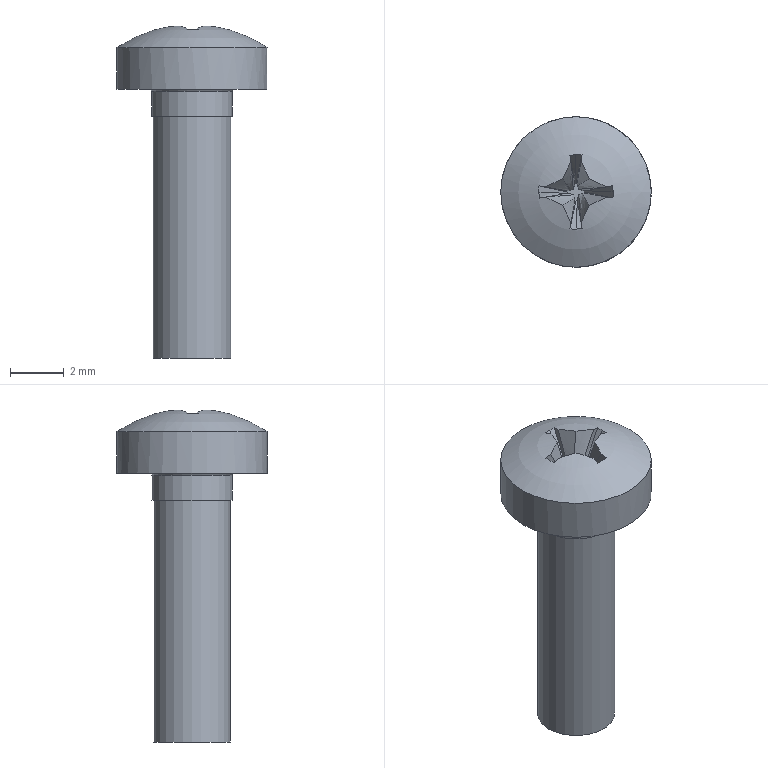Part | NX | features SKETCH 3, DATUM_CSYS 2, DATUM_PLANE 2, FSET 1, LINE 1, META 1, SKIN 1, SWP104 1, SYMBOLIC_THREAD 1, THREADS 1 | 1 solid | 33 faces | box 5.6 x 5.6 x 12.351 mm | volume 111.736 mm3 | spline 20 | plane 8 | cylinder 3 | sphere 1 | torus 1 | commonest cylinder face diameters 2.874 x1 3 x1 5.6 x1
STEP:
#1=CARTESIAN_POINT('',(-2.8,0.,1.542));
#2=VERTEX_POINT('',#1);
#3=CARTESIAN_POINT('',(0.,0.,1.542));
#4=DIRECTION('',(0.,0.,-1.));
#5=DIRECTION('',(-1.,0.,0.));
#6=AXIS2_PLACEMENT_3D('',#3,#4,#5);
#7=CIRCLE('',#6,2.8);
#8=EDGE_CURVE('',#2,#2,#7,.T.);
#9=ORIENTED_EDGE('',*,*,#8,.F.);
#10=EDGE_LOOP('',(#9));
#11=FACE_BOUND('',#10,.T.);
#12=CARTESIAN_POINT('',(-0.4967,0.4916,2.351));
#13=VERTEX_POINT('',#12);
#14=CARTESIAN_POINT('',(-1.137,0.1895,2.265));
#15=VERTEX_POINT('',#14);
#16=CARTESIAN_POINT('',(-0.4967,0.4916,2.351));
#17=CARTESIAN_POINT('',(-0.7133,0.3939,2.339));
#18=CARTESIAN_POINT('',(-0.9272,0.2926,2.31));
#19=CARTESIAN_POINT('',(-1.137,0.1895,2.265));
#20=B_SPLINE_CURVE_WITH_KNOTS('',3,(#16,#17,#18,#19),.UNSPECIFIED.,.F.,.F.,(4,4),(0.,0.0007137),.UNSPECIFIED.);
#21=EDGE_CURVE('',#13,#15,#20,.T.);
#22=ORIENTED_EDGE('',*,*,#21,.F.);
#23=CARTESIAN_POINT('',(-0.1932,1.124,2.268));
#24=VERTEX_POINT('',#23);
#25=CARTESIAN_POINT('',(-0.1932,1.124,2.268));
#26=CARTESIAN_POINT('',(-0.2989,0.9182,2.312));
#27=CARTESIAN_POINT('',(-0.3995,0.7062,2.339));
#28=CARTESIAN_POINT('',(-0.4967,0.4916,2.351));
#29=B_SPLINE_CURVE_WITH_KNOTS('',3,(#25,#26,#27,#28),.UNSPECIFIED.,.F.,.F.,(4,4),(0.,0.0007074),.UNSPECIFIED.);
#30=EDGE_CURVE('',#24,#13,#29,.T.);
#31=ORIENTED_EDGE('',*,*,#30,.F.);
#32=CARTESIAN_POINT('',(-0.2285,1.371,2.203));
#33=VERTEX_POINT('',#32);
#34=CARTESIAN_POINT('',(-0.2285,1.371,2.203));
#35=CARTESIAN_POINT('',(-0.2178,1.289,2.227));
#36=CARTESIAN_POINT('',(-0.2059,1.207,2.249));
#37=CARTESIAN_POINT('',(-0.1932,1.124,2.268));
#38=B_SPLINE_CURVE_WITH_KNOTS('',3,(#34,#35,#36,#37),.UNSPECIFIED.,.F.,.F.,(4,4),(0.,0.0002572),.UNSPECIFIED.);
#39=EDGE_CURVE('',#33,#24,#38,.T.);
#40=ORIENTED_EDGE('',*,*,#39,.F.);
#41=CARTESIAN_POINT('',(-0.005049,1.379,2.206));
#42=VERTEX_POINT('',#41);
#43=CARTESIAN_POINT('',(-0.005049,1.379,2.206));
#44=CARTESIAN_POINT('',(-0.07956,1.377,2.207));
#45=CARTESIAN_POINT('',(-0.1541,1.374,2.205));
#46=CARTESIAN_POINT('',(-0.2285,1.371,2.203));
#47=B_SPLINE_CURVE_WITH_KNOTS('',3,(#43,#44,#45,#46),.UNSPECIFIED.,.F.,.F.,(4,4),(0.,0.0002236),.UNSPECIFIED.);
#48=EDGE_CURVE('',#42,#33,#47,.T.);
#49=ORIENTED_EDGE('',*,*,#48,.F.);
#50=CARTESIAN_POINT('',(0.2242,1.376,2.202));
#51=VERTEX_POINT('',#50);
#52=CARTESIAN_POINT('',(0.,-1.169,-1.87));
#53=DIRECTION('',(0.,-0.848,0.53));
#54=DIRECTION('',(0.,-0.53,-0.848));
#55=AXIS2_PLACEMENT_3D('',#52,#53,#54);
#56=CIRCLE('',#55,4.806);
#57=EDGE_CURVE('',#51,#42,#56,.T.);
#58=ORIENTED_EDGE('',*,*,#57,.F.);
#59=CARTESIAN_POINT('',(0.1895,1.137,2.265));
#60=VERTEX_POINT('',#59);
#61=CARTESIAN_POINT('',(0.1895,1.137,2.265));
#62=CARTESIAN_POINT('',(0.2017,1.217,2.246));
#63=CARTESIAN_POINT('',(0.2134,1.297,2.225));
#64=CARTESIAN_POINT('',(0.2242,1.376,2.202));
#65=B_SPLINE_CURVE_WITH_KNOTS('',3,(#61,#62,#63,#64),.UNSPECIFIED.,.F.,.F.,(4,4),(0.,0.0002499),.UNSPECIFIED.);
#66=EDGE_CURVE('',#60,#51,#65,.T.);
#67=ORIENTED_EDGE('',*,*,#66,.F.);
#68=CARTESIAN_POINT('',(0.4916,0.4967,2.351));
#69=VERTEX_POINT('',#68);
#70=CARTESIAN_POINT('',(0.4916,0.4967,2.351));
#71=CARTESIAN_POINT('',(0.3939,0.7133,2.339));
#72=CARTESIAN_POINT('',(0.2926,0.9272,2.31));
#73=CARTESIAN_POINT('',(0.1895,1.137,2.265));
#74=B_SPLINE_CURVE_WITH_KNOTS('',3,(#70,#71,#72,#73),.UNSPECIFIED.,.F.,.F.,(4,4),(0.,0.0007137),.UNSPECIFIED.);
#75=EDGE_CURVE('',#69,#60,#74,.T.);
#76=ORIENTED_EDGE('',*,*,#75,.F.);
#77=CARTESIAN_POINT('',(1.124,0.1932,2.268));
#78=VERTEX_POINT('',#77);
#79=CARTESIAN_POINT('',(1.124,0.1932,2.268));
#80=CARTESIAN_POINT('',(0.9182,0.2989,2.312));
#81=CARTESIAN_POINT('',(0.7062,0.3995,2.339));
#82=CARTESIAN_POINT('',(0.4916,0.4967,2.351));
#83=B_SPLINE_CURVE_WITH_KNOTS('',3,(#79,#80,#81,#82),.UNSPECIFIED.,.F.,.F.,(4,4),(0.,0.0007074),.UNSPECIFIED.);
#84=EDGE_CURVE('',#78,#69,#83,.T.);
#85=ORIENTED_EDGE('',*,*,#84,.F.);
#86=CARTESIAN_POINT('',(1.371,0.2285,2.203));
#87=VERTEX_POINT('',#86);
#88=CARTESIAN_POINT('',(1.371,0.2285,2.203));
#89=CARTESIAN_POINT('',(1.289,0.2178,2.227));
#90=CARTESIAN_POINT('',(1.207,0.2059,2.249));
#91=CARTESIAN_POINT('',(1.124,0.1932,2.268));
#92=B_SPLINE_CURVE_WITH_KNOTS('',3,(#88,#89,#90,#91),.UNSPECIFIED.,.F.,.F.,(4,4),(0.,0.0002572),.UNSPECIFIED.);
#93=EDGE_CURVE('',#87,#78,#92,.T.);
#94=ORIENTED_EDGE('',*,*,#93,.F.);
#95=CARTESIAN_POINT('',(1.379,0.005049,2.206));
#96=VERTEX_POINT('',#95);
#97=CARTESIAN_POINT('',(1.379,0.005049,2.206));
#98=CARTESIAN_POINT('',(1.377,0.07956,2.207));
#99=CARTESIAN_POINT('',(1.374,0.1541,2.205));
#100=CARTESIAN_POINT('',(1.371,0.2285,2.203));
#101=B_SPLINE_CURVE_WITH_KNOTS('',3,(#97,#98,#99,#100),.UNSPECIFIED.,.F.,.F.,(4,4),(0.,0.0002236),.UNSPECIFIED.);
#102=EDGE_CURVE('',#96,#87,#101,.T.);
#103=ORIENTED_EDGE('',*,*,#102,.F.);
#104=CARTESIAN_POINT('',(1.376,-0.2242,2.202));
#105=VERTEX_POINT('',#104);
#106=CARTESIAN_POINT('',(-1.169,0.,-1.87));
#107=DIRECTION('',(-0.848,0.,0.53));
#108=DIRECTION('',(0.53,0.,0.848));
#109=AXIS2_PLACEMENT_3D('',#106,#107,#108);
#110=CIRCLE('',#109,4.806);
#111=EDGE_CURVE('',#105,#96,#110,.T.);
#112=ORIENTED_EDGE('',*,*,#111,.F.);
#113=CARTESIAN_POINT('',(1.137,-0.1895,2.265));
#114=VERTEX_POINT('',#113);
#115=CARTESIAN_POINT('',(1.137,-0.1895,2.265));
#116=CARTESIAN_POINT('',(1.217,-0.2017,2.246));
#117=CARTESIAN_POINT('',(1.297,-0.2134,2.225));
#118=CARTESIAN_POINT('',(1.376,-0.2242,2.202));
#119=B_SPLINE_CURVE_WITH_KNOTS('',3,(#115,#116,#117,#118),.UNSPECIFIED.,.F.,.F.,(4,4),(0.,0.0002499),.UNSPECIFIED.);
#120=EDGE_CURVE('',#114,#105,#119,.T.);
#121=ORIENTED_EDGE('',*,*,#120,.F.);
#122=CARTESIAN_POINT('',(0.4967,-0.4916,2.351));
#123=VERTEX_POINT('',#122);
#124=CARTESIAN_POINT('',(0.4967,-0.4916,2.351));
#125=CARTESIAN_POINT('',(0.7133,-0.3939,2.339));
#126=CARTESIAN_POINT('',(0.9272,-0.2926,2.31));
#127=CARTESIAN_POINT('',(1.137,-0.1895,2.265));
#128=B_SPLINE_CURVE_WITH_KNOTS('',3,(#124,#125,#126,#127),.UNSPECIFIED.,.F.,.F.,(4,4),(0.,0.0007137),.UNSPECIFIED.);
#129=EDGE_CURVE('',#123,#114,#128,.T.);
#130=ORIENTED_EDGE('',*,*,#129,.F.);
#131=CARTESIAN_POINT('',(0.1932,-1.124,2.268));
#132=VERTEX_POINT('',#131);
#133=CARTESIAN_POINT('',(0.1932,-1.124,2.268));
#134=CARTESIAN_POINT('',(0.2989,-0.9182,2.312));
#135=CARTESIAN_POINT('',(0.3995,-0.7062,2.339));
#136=CARTESIAN_POINT('',(0.4967,-0.4916,2.351));
#137=B_SPLINE_CURVE_WITH_KNOTS('',3,(#133,#134,#135,#136),.UNSPECIFIED.,.F.,.F.,(4,4),(0.,0.0007074),.UNSPECIFIED.);
#138=EDGE_CURVE('',#132,#123,#137,.T.);
#139=ORIENTED_EDGE('',*,*,#138,.F.);
#140=CARTESIAN_POINT('',(0.2285,-1.371,2.203));
#141=VERTEX_POINT('',#140);
#142=CARTESIAN_POINT('',(0.2285,-1.371,2.203));
#143=CARTESIAN_POINT('',(0.2178,-1.289,2.227));
#144=CARTESIAN_POINT('',(0.2059,-1.207,2.249));
#145=CARTESIAN_POINT('',(0.1932,-1.124,2.268));
#146=B_SPLINE_CURVE_WITH_KNOTS('',3,(#142,#143,#144,#145),.UNSPECIFIED.,.F.,.F.,(4,4),(0.,0.0002572),.UNSPECIFIED.);
#147=EDGE_CURVE('',#141,#132,#146,.T.);
#148=ORIENTED_EDGE('',*,*,#147,.F.);
#149=CARTESIAN_POINT('',(0.005049,-1.379,2.206));
#150=VERTEX_POINT('',#149);
#151=CARTESIAN_POINT('',(0.005049,-1.379,2.206));
#152=CARTESIAN_POINT('',(0.07956,-1.377,2.207));
#153=CARTESIAN_POINT('',(0.1541,-1.374,2.205));
#154=CARTESIAN_POINT('',(0.2285,-1.371,2.203));
#155=B_SPLINE_CURVE_WITH_KNOTS('',3,(#151,#152,#153,#154),.UNSPECIFIED.,.F.,.F.,(4,4),(0.,0.0002236),.UNSPECIFIED.);
#156=EDGE_CURVE('',#150,#141,#155,.T.);
#157=ORIENTED_EDGE('',*,*,#156,.F.);
#158=CARTESIAN_POINT('',(-0.2242,-1.376,2.202));
#159=VERTEX_POINT('',#158);
#160=CARTESIAN_POINT('',(0.,1.169,-1.87));
#161=DIRECTION('',(0.,0.848,0.53));
#162=DIRECTION('',(0.,-0.53,0.848));
#163=AXIS2_PLACEMENT_3D('',#160,#161,#162);
#164=CIRCLE('',#163,4.806);
#165=EDGE_CURVE('',#159,#150,#164,.T.);
#166=ORIENTED_EDGE('',*,*,#165,.F.);
#167=CARTESIAN_POINT('',(-0.1895,-1.137,2.265));
#168=VERTEX_POINT('',#167);
#169=CARTESIAN_POINT('',(-0.1895,-1.137,2.265));
#170=CARTESIAN_POINT('',(-0.2017,-1.217,2.246));
#171=CARTESIAN_POINT('',(-0.2134,-1.297,2.225));
#172=CARTESIAN_POINT('',(-0.2242,-1.376,2.202));
#173=B_SPLINE_CURVE_WITH_KNOTS('',3,(#169,#170,#171,#172),.UNSPECIFIED.,.F.,.F.,(4,4),(0.,0.0002499),.UNSPECIFIED.);
#174=EDGE_CURVE('',#168,#159,#173,.T.);
#175=ORIENTED_EDGE('',*,*,#174,.F.);
#176=CARTESIAN_POINT('',(-0.4916,-0.4967,2.351));
#177=VERTEX_POINT('',#176);
#178=CARTESIAN_POINT('',(-0.4916,-0.4967,2.351));
#179=CARTESIAN_POINT('',(-0.3939,-0.7133,2.339));
#180=CARTESIAN_POINT('',(-0.2926,-0.9272,2.31));
#181=CARTESIAN_POINT('',(-0.1895,-1.137,2.265));
#182=B_SPLINE_CURVE_WITH_KNOTS('',3,(#178,#179,#180,#181),.UNSPECIFIED.,.F.,.F.,(4,4),(0.,0.0007137),.UNSPECIFIED.);
#183=EDGE_CURVE('',#177,#168,#182,.T.);
#184=ORIENTED_EDGE('',*,*,#183,.F.);
#185=CARTESIAN_POINT('',(-1.124,-0.1932,2.268));
#186=VERTEX_POINT('',#185);
#187=CARTESIAN_POINT('',(-1.124,-0.1932,2.268));
#188=CARTESIAN_POINT('',(-0.9182,-0.2989,2.312));
#189=CARTESIAN_POINT('',(-0.7062,-0.3995,2.339));
#190=CARTESIAN_POINT('',(-0.4916,-0.4967,2.351));
#191=B_SPLINE_CURVE_WITH_KNOTS('',3,(#187,#188,#189,#190),.UNSPECIFIED.,.F.,.F.,(4,4),(0.,0.0007074),.UNSPECIFIED.);
#192=EDGE_CURVE('',#186,#177,#191,.T.);
#193=ORIENTED_EDGE('',*,*,#192,.F.);
#194=CARTESIAN_POINT('',(-1.371,-0.2285,2.203));
#195=VERTEX_POINT('',#194);
#196=CARTESIAN_POINT('',(-1.371,-0.2285,2.203));
#197=CARTESIAN_POINT('',(-1.289,-0.2178,2.227));
#198=CARTESIAN_POINT('',(-1.207,-0.2059,2.249));
#199=CARTESIAN_POINT('',(-1.124,-0.1932,2.268));
#200=B_SPLINE_CURVE_WITH_KNOTS('',3,(#196,#197,#198,#199),.UNSPECIFIED.,.F.,.F.,(4,4),(0.,0.0002572),.UNSPECIFIED.);
#201=EDGE_CURVE('',#195,#186,#200,.T.);
#202=ORIENTED_EDGE('',*,*,#201,.F.);
#203=CARTESIAN_POINT('',(-1.379,-0.005049,2.206));
#204=VERTEX_POINT('',#203);
#205=CARTESIAN_POINT('',(-1.379,-0.005049,2.206));
#206=CARTESIAN_POINT('',(-1.377,-0.07956,2.207));
#207=CARTESIAN_POINT('',(-1.374,-0.1541,2.205));
#208=CARTESIAN_POINT('',(-1.371,-0.2285,2.203));
#209=B_SPLINE_CURVE_WITH_KNOTS('',3,(#205,#206,#207,#208),.UNSPECIFIED.,.F.,.F.,(4,4),(0.,0.0002236),.UNSPECIFIED.);
#210=EDGE_CURVE('',#204,#195,#209,.T.);
#211=ORIENTED_EDGE('',*,*,#210,.F.);
#212=CARTESIAN_POINT('',(-1.376,0.2242,2.202));
#213=VERTEX_POINT('',#212);
#214=CARTESIAN_POINT('',(1.169,0.,-1.87));
#215=DIRECTION('',(0.848,0.,0.53));
#216=DIRECTION('',(0.53,0.,-0.848));
#217=AXIS2_PLACEMENT_3D('',#214,#215,#216);
#218=CIRCLE('',#217,4.806);
#219=EDGE_CURVE('',#213,#204,#218,.T.);
#220=ORIENTED_EDGE('',*,*,#219,.F.);
#221=CARTESIAN_POINT('',(-1.137,0.1895,2.265));
#222=CARTESIAN_POINT('',(-1.217,0.2017,2.246));
#223=CARTESIAN_POINT('',(-1.297,0.2134,2.225));
#224=CARTESIAN_POINT('',(-1.376,0.2242,2.202));
#225=B_SPLINE_CURVE_WITH_KNOTS('',3,(#221,#222,#223,#224),.UNSPECIFIED.,.F.,.F.,(4,4),(0.,0.0002499),.UNSPECIFIED.);
#226=EDGE_CURVE('',#15,#213,#225,.T.);
#227=ORIENTED_EDGE('',*,*,#226,.F.);
#228=EDGE_LOOP('',(#22,#31,#40,#49,#58,#67,#76,#85,#94,#103,#112,#121,#130,#139,#148,#157,#166,#175,#184,#193,#202,#211,#220,#227));
#229=FACE_BOUND('',#228,.T.);
#230=CARTESIAN_POINT('',(0.,0.,-2.6));
#231=DIRECTION('',(0.,0.,-1.));
#232=DIRECTION('',(1.,0.,0.));
#233=AXIS2_PLACEMENT_3D('',#230,#231,#232);
#234=SPHERICAL_SURFACE('',#233,5.);
#235=ADVANCED_FACE('',(#11,#229),#234,.T.);
#236=CARTESIAN_POINT('',(-2.8,0.,0.));
#237=VERTEX_POINT('',#236);
#238=CARTESIAN_POINT('',(0.,0.,0.));
#239=DIRECTION('',(0.,0.,-1.));
#240=DIRECTION('',(-1.,0.,0.));
#241=AXIS2_PLACEMENT_3D('',#238,#239,#240);
#242=CIRCLE('',#241,2.8);
#243=EDGE_CURVE('',#237,#237,#242,.T.);
#244=ORIENTED_EDGE('',*,*,#243,.F.);
#245=EDGE_LOOP('',(#244));
#246=FACE_BOUND('',#245,.T.);
#247=ORIENTED_EDGE('',*,*,#8,.T.);
#248=EDGE_LOOP('',(#247));
#249=FACE_BOUND('',#248,.T.);
#250=CARTESIAN_POINT('',(0.,0.,0.));
#251=DIRECTION('',(0.,0.,-1.));
#252=DIRECTION('',(-1.,0.,0.));
#253=AXIS2_PLACEMENT_3D('',#250,#251,#252);
#254=CYLINDRICAL_SURFACE('',#253,2.8);
#255=ADVANCED_FACE('',(#246,#249),#254,.T.);
#256=CARTESIAN_POINT('',(-1.6,0.,0.));
#257=VERTEX_POINT('',#256);
#258=CARTESIAN_POINT('',(0.,0.,0.));
#259=DIRECTION('',(0.,0.,-1.));
#260=DIRECTION('',(-1.,0.,0.));
#261=AXIS2_PLACEMENT_3D('',#258,#259,#260);
#262=CIRCLE('',#261,1.6);
#263=EDGE_CURVE('',#257,#257,#262,.T.);
#264=ORIENTED_EDGE('',*,*,#263,.F.);
#265=EDGE_LOOP('',(#264));
#266=FACE_BOUND('',#265,.T.);
#267=ORIENTED_EDGE('',*,*,#243,.T.);
#268=EDGE_LOOP('',(#267));
#269=FACE_BOUND('',#268,.T.);
#270=CARTESIAN_POINT('',(2.8,0.,0.));
#271=DIRECTION('',(0.,0.,1.));
#272=DIRECTION('',(1.,0.,0.));
#273=AXIS2_PLACEMENT_3D('',#270,#271,#272);
#274=PLANE('',#273);
#275=ADVANCED_FACE('',(#266,#269),#274,.F.);
#276=CARTESIAN_POINT('',(-1.5,0.,-0.1));
#277=VERTEX_POINT('',#276);
#278=CARTESIAN_POINT('',(0.,0.,-0.1));
#279=DIRECTION('',(0.,0.,-1.));
#280=DIRECTION('',(-1.,0.,0.));
#281=AXIS2_PLACEMENT_3D('',#278,#279,#280);
#282=CIRCLE('',#281,1.5);
#283=EDGE_CURVE('',#277,#277,#282,.T.);
#284=ORIENTED_EDGE('',*,*,#283,.F.);
#285=EDGE_LOOP('',(#284));
#286=FACE_BOUND('',#285,.T.);
#287=ORIENTED_EDGE('',*,*,#263,.T.);
#288=EDGE_LOOP('',(#287));
#289=FACE_BOUND('',#288,.T.);
#290=CARTESIAN_POINT('',(0.,0.,-0.1));
#291=DIRECTION('',(0.,0.,-1.));
#292=DIRECTION('',(-1.,0.,0.));
#293=AXIS2_PLACEMENT_3D('',#290,#291,#292);
#294=TOROIDAL_SURFACE('',#293,1.6,0.1);
#295=ADVANCED_FACE('',(#286,#289),#294,.F.);
#296=CARTESIAN_POINT('',(-1.5,0.,-1.));
#297=VERTEX_POINT('',#296);
#298=CARTESIAN_POINT('',(0.,0.,-1.));
#299=DIRECTION('',(0.,0.,-1.));
#300=DIRECTION('',(-1.,0.,0.));
#301=AXIS2_PLACEMENT_3D('',#298,#299,#300);
#302=CIRCLE('',#301,1.5);
#303=EDGE_CURVE('',#297,#297,#302,.T.);
#304=ORIENTED_EDGE('',*,*,#303,.F.);
#305=EDGE_LOOP('',(#304));
#306=FACE_BOUND('',#305,.T.);
#307=ORIENTED_EDGE('',*,*,#283,.T.);
#308=EDGE_LOOP('',(#307));
#309=FACE_BOUND('',#308,.T.);
#310=CARTESIAN_POINT('',(0.,0.,0.));
#311=DIRECTION('',(0.,0.,-1.));
#312=DIRECTION('',(-1.,0.,0.));
#313=AXIS2_PLACEMENT_3D('',#310,#311,#312);
#314=CYLINDRICAL_SURFACE('',#313,1.5);
#315=ADVANCED_FACE('',(#306,#309),#314,.T.);
#316=CARTESIAN_POINT('',(-1.437,0.,-1.));
#317=VERTEX_POINT('',#316);
#318=CARTESIAN_POINT('',(0.,0.,-1.));
#319=DIRECTION('',(0.,0.,-1.));
#320=DIRECTION('',(-1.,0.,0.));
#321=AXIS2_PLACEMENT_3D('',#318,#319,#320);
#322=CIRCLE('',#321,1.437);
#323=EDGE_CURVE('',#317,#317,#322,.T.);
#324=ORIENTED_EDGE('',*,*,#323,.F.);
#325=EDGE_LOOP('',(#324));
#326=FACE_BOUND('',#325,.T.);
#327=ORIENTED_EDGE('',*,*,#303,.T.);
#328=EDGE_LOOP('',(#327));
#329=FACE_BOUND('',#328,.T.);
#330=CARTESIAN_POINT('',(1.5,0.,-1.));
#331=DIRECTION('',(0.,0.,1.));
#332=DIRECTION('',(1.,0.,0.));
#333=AXIS2_PLACEMENT_3D('',#330,#331,#332);
#334=PLANE('',#333);
#335=ADVANCED_FACE('',(#326,#329),#334,.F.);
#336=CARTESIAN_POINT('',(-1.437,0.,-10.));
#337=VERTEX_POINT('',#336);
#338=CARTESIAN_POINT('',(0.,0.,-10.));
#339=DIRECTION('',(0.,0.,-1.));
#340=DIRECTION('',(-1.,0.,0.));
#341=AXIS2_PLACEMENT_3D('',#338,#339,#340);
#342=CIRCLE('',#341,1.437);
#343=EDGE_CURVE('',#337,#337,#342,.T.);
#344=ORIENTED_EDGE('',*,*,#343,.F.);
#345=EDGE_LOOP('',(#344));
#346=FACE_BOUND('',#345,.T.);
#347=ORIENTED_EDGE('',*,*,#323,.T.);
#348=EDGE_LOOP('',(#347));
#349=FACE_BOUND('',#348,.T.);
#350=CARTESIAN_POINT('',(0.,0.,0.));
#351=DIRECTION('',(0.,0.,-1.));
#352=DIRECTION('',(-1.,0.,0.));
#353=AXIS2_PLACEMENT_3D('',#350,#351,#352);
#354=CYLINDRICAL_SURFACE('',#353,1.437);
#355=ADVANCED_FACE('',(#346,#349),#354,.T.);
#356=ORIENTED_EDGE('',*,*,#343,.T.);
#357=EDGE_LOOP('',(#356));
#358=FACE_BOUND('',#357,.T.);
#359=CARTESIAN_POINT('',(1.437,0.,-10.));
#360=DIRECTION('',(0.,0.,1.));
#361=DIRECTION('',(1.,0.,0.));
#362=AXIS2_PLACEMENT_3D('',#359,#360,#361);
#363=PLANE('',#362);
#364=ADVANCED_FACE('',(#358),#363,.F.);
#365=ORIENTED_EDGE('',*,*,#21,.T.);
#366=CARTESIAN_POINT('',(-0.3,0.05,0.48));
#367=VERTEX_POINT('',#366);
#368=CARTESIAN_POINT('',(-1.2,0.2,2.4));
#369=CARTESIAN_POINT('',(-0.3,0.05,0.48));
#370=B_SPLINE_CURVE_WITH_KNOTS('',1,(#368,#369),.UNSPECIFIED.,.F.,.F.,(2,2),(0.,1.),.PIECEWISE_BEZIER_KNOTS.);
#371=EDGE_CURVE('',#15,#367,#370,.T.);
#372=ORIENTED_EDGE('',*,*,#371,.T.);
#373=CARTESIAN_POINT('',(-0.24,0.04,0.48));
#374=VERTEX_POINT('',#373);
#375=CARTESIAN_POINT('',(-0.3,0.05,0.48));
#376=CARTESIAN_POINT('',(-0.28,0.04667,0.48));
#377=CARTESIAN_POINT('',(-0.26,0.04333,0.48));
#378=CARTESIAN_POINT('',(-0.24,0.04,0.48));
#379=B_SPLINE_CURVE_WITH_KNOTS('',3,(#375,#376,#377,#378),.UNSPECIFIED.,.F.,.F.,(4,4),(0.,1.),.UNSPECIFIED.);
#380=EDGE_CURVE('',#367,#374,#379,.T.);
#381=ORIENTED_EDGE('',*,*,#380,.T.);
#382=CARTESIAN_POINT('',(-0.5034,0.5034,2.4));
#383=CARTESIAN_POINT('',(-0.24,0.04,0.48));
#384=B_SPLINE_CURVE_WITH_KNOTS('',1,(#382,#383),.UNSPECIFIED.,.F.,.F.,(2,2),(0.,1.),.PIECEWISE_BEZIER_KNOTS.);
#385=EDGE_CURVE('',#13,#374,#384,.T.);
#386=ORIENTED_EDGE('',*,*,#385,.F.);
#387=EDGE_LOOP('',(#365,#372,#381,#386));
#388=FACE_BOUND('',#387,.T.);
#389=CARTESIAN_POINT('',(-0.4982,0.4943,2.362));
#390=CARTESIAN_POINT('',(-0.24,0.04,0.48));
#391=CARTESIAN_POINT('',(-1.182,0.197,2.362));
#392=CARTESIAN_POINT('',(-0.3,0.05,0.48));
#393=B_SPLINE_SURFACE_WITH_KNOTS('',1,1,((#389,#390),(#391,#392)),.RULED_SURF.,.F.,.F.,.F.,(2,2),(2,2),(0.,1.),(0.01971,1.),.PIECEWISE_BEZIER_KNOTS.);
#394=ADVANCED_FACE('',(#388),#393,.T.);
#395=ORIENTED_EDGE('',*,*,#30,.T.);
#396=ORIENTED_EDGE('',*,*,#385,.T.);
#397=CARTESIAN_POINT('',(-0.1007,0.1007,0.48));
#398=VERTEX_POINT('',#397);
#399=CARTESIAN_POINT('',(-0.24,0.04,0.48));
#400=CARTESIAN_POINT('',(-0.1936,0.06023,0.48));
#401=CARTESIAN_POINT('',(-0.1471,0.08046,0.48));
#402=CARTESIAN_POINT('',(-0.1007,0.1007,0.48));
#403=B_SPLINE_CURVE_WITH_KNOTS('',3,(#399,#400,#401,#402),.UNSPECIFIED.,.F.,.F.,(4,4),(0.,1.),.UNSPECIFIED.);
#404=EDGE_CURVE('',#374,#398,#403,.T.);
#405=ORIENTED_EDGE('',*,*,#404,.T.);
#406=CARTESIAN_POINT('',(-0.2,1.2,2.4));
#407=CARTESIAN_POINT('',(-0.1007,0.1007,0.48));
#408=B_SPLINE_CURVE_WITH_KNOTS('',1,(#406,#407),.UNSPECIFIED.,.F.,.F.,(2,2),(0.,1.),.PIECEWISE_BEZIER_KNOTS.);
#409=EDGE_CURVE('',#24,#398,#408,.T.);
#410=ORIENTED_EDGE('',*,*,#409,.F.);
#411=EDGE_LOOP('',(#395,#396,#405,#410));
#412=FACE_BOUND('',#411,.T.);
#413=CARTESIAN_POINT('',(-0.198,1.178,2.362));
#414=CARTESIAN_POINT('',(-0.1007,0.1007,0.48));
#415=CARTESIAN_POINT('',(-0.4982,0.4943,2.362));
#416=CARTESIAN_POINT('',(-0.24,0.04,0.48));
#417=B_SPLINE_SURFACE_WITH_KNOTS('',1,1,((#413,#414),(#415,#416)),.RULED_SURF.,.F.,.F.,.F.,(2,2),(2,2),(0.,1.),(0.01971,1.),.PIECEWISE_BEZIER_KNOTS.);
#418=ADVANCED_FACE('',(#412),#417,.T.);
#419=ORIENTED_EDGE('',*,*,#39,.T.);
#420=ORIENTED_EDGE('',*,*,#409,.T.);
#421=CARTESIAN_POINT('',(-0.04,0.24,0.48));
#422=VERTEX_POINT('',#421);
#423=CARTESIAN_POINT('',(-0.1007,0.1007,0.48));
#424=CARTESIAN_POINT('',(-0.08046,0.1471,0.48));
#425=CARTESIAN_POINT('',(-0.06023,0.1936,0.48));
#426=CARTESIAN_POINT('',(-0.04,0.24,0.48));
#427=B_SPLINE_CURVE_WITH_KNOTS('',3,(#423,#424,#425,#426),.UNSPECIFIED.,.F.,.F.,(4,4),(0.,1.),.UNSPECIFIED.);
#428=EDGE_CURVE('',#398,#422,#427,.T.);
#429=ORIENTED_EDGE('',*,*,#428,.T.);
#430=CARTESIAN_POINT('',(-0.25,1.5,2.4));
#431=CARTESIAN_POINT('',(-0.04,0.24,0.48));
#432=B_SPLINE_CURVE_WITH_KNOTS('',1,(#430,#431),.UNSPECIFIED.,.F.,.F.,(2,2),(0.,1.),.PIECEWISE_BEZIER_KNOTS.);
#433=EDGE_CURVE('',#33,#422,#432,.T.);
#434=ORIENTED_EDGE('',*,*,#433,.F.);
#435=EDGE_LOOP('',(#419,#420,#429,#434));
#436=FACE_BOUND('',#435,.T.);
#437=CARTESIAN_POINT('',(-0.2367,1.42,2.279));
#438=CARTESIAN_POINT('',(-0.04,0.24,0.48));
#439=CARTESIAN_POINT('',(-0.1937,1.131,2.279));
#440=CARTESIAN_POINT('',(-0.1007,0.1007,0.48));
#441=B_SPLINE_SURFACE_WITH_KNOTS('',1,1,((#437,#438),(#439,#440)),.RULED_SURF.,.F.,.F.,.F.,(2,2),(2,2),(0.,1.),(0.06312,1.),.PIECEWISE_BEZIER_KNOTS.);
#442=ADVANCED_FACE('',(#436),#441,.T.);
#443=ORIENTED_EDGE('',*,*,#48,.T.);
#444=ORIENTED_EDGE('',*,*,#433,.T.);
#445=CARTESIAN_POINT('',(-0.05,0.3,0.48));
#446=VERTEX_POINT('',#445);
#447=CARTESIAN_POINT('',(-0.04,0.24,0.48));
#448=CARTESIAN_POINT('',(-0.04333,0.26,0.48));
#449=CARTESIAN_POINT('',(-0.04667,0.28,0.48));
#450=CARTESIAN_POINT('',(-0.05,0.3,0.48));
#451=B_SPLINE_CURVE_WITH_KNOTS('',3,(#447,#448,#449,#450),.UNSPECIFIED.,.F.,.F.,(4,4),(0.,1.),.UNSPECIFIED.);
#452=EDGE_CURVE('',#422,#446,#451,.T.);
#453=ORIENTED_EDGE('',*,*,#452,.T.);
#454=CARTESIAN_POINT('',(-0.025,0.9,1.44));
#455=DIRECTION('',(-0.02208,-0.5299,-0.8478));
#456=VECTOR('',#455,1000.);
#457=LINE('',#454,#456);
#458=EDGE_CURVE('',#42,#446,#457,.T.);
#459=ORIENTED_EDGE('',*,*,#458,.F.);
#460=EDGE_LOOP('',(#443,#444,#453,#459));
#461=FACE_BOUND('',#460,.T.);
#462=CARTESIAN_POINT('',(-0.004776,1.385,2.217));
#463=CARTESIAN_POINT('',(-0.05,0.3,0.48));
#464=CARTESIAN_POINT('',(-0.2299,1.38,2.217));
#465=CARTESIAN_POINT('',(-0.04,0.24,0.48));
#466=B_SPLINE_SURFACE_WITH_KNOTS('',1,1,((#462,#463),(#464,#465)),.RULED_SURF.,.F.,.F.,.F.,(2,2),(2,2),(0.,1.),(0.09552,1.),.PIECEWISE_BEZIER_KNOTS.);
#467=ADVANCED_FACE('',(#461),#466,.T.);
#468=ORIENTED_EDGE('',*,*,#57,.T.);
#469=ORIENTED_EDGE('',*,*,#458,.T.);
#470=CARTESIAN_POINT('',(0.,0.3,0.48));
#471=VERTEX_POINT('',#470);
#472=CARTESIAN_POINT('',(-0.025,0.3,0.48));
#473=DIRECTION('',(-1.,0.,0.));
#474=VECTOR('',#473,1000.);
#475=LINE('',#472,#474);
#476=EDGE_CURVE('',#471,#446,#475,.T.);
#477=ORIENTED_EDGE('',*,*,#476,.F.);
#478=CARTESIAN_POINT('',(0.25,1.5,2.4));
#479=CARTESIAN_POINT('',(0.,0.3,0.48));
#480=B_SPLINE_CURVE_WITH_KNOTS('',1,(#478,#479),.UNSPECIFIED.,.F.,.F.,(2,2),(0.,1.),.PIECEWISE_BEZIER_KNOTS.);
#481=EDGE_CURVE('',#51,#471,#480,.T.);
#482=ORIENTED_EDGE('',*,*,#481,.F.);
#483=EDGE_LOOP('',(#468,#469,#477,#482));
#484=FACE_BOUND('',#483,.T.);
#485=CARTESIAN_POINT('',(0.125,0.9,1.44));
#486=DIRECTION('',(0.,-0.848,0.53));
#487=DIRECTION('',(0.,-0.53,-0.848));
#488=AXIS2_PLACEMENT_3D('',#485,#486,#487);
#489=PLANE('',#488);
#490=ADVANCED_FACE('',(#484),#489,.T.);
#491=ORIENTED_EDGE('',*,*,#66,.T.);
#492=ORIENTED_EDGE('',*,*,#481,.T.);
#493=CARTESIAN_POINT('',(0.05,0.3,0.48));
#494=VERTEX_POINT('',#493);
#495=CARTESIAN_POINT('',(0.,0.3,0.48));
#496=CARTESIAN_POINT('',(0.01667,0.3,0.48));
#497=CARTESIAN_POINT('',(0.03333,0.3,0.48));
#498=CARTESIAN_POINT('',(0.05,0.3,0.48));
#499=B_SPLINE_CURVE_WITH_KNOTS('',3,(#495,#496,#497,#498),.UNSPECIFIED.,.F.,.F.,(4,4),(0.,1.),.UNSPECIFIED.);
#500=EDGE_CURVE('',#471,#494,#499,.T.);
#501=ORIENTED_EDGE('',*,*,#500,.T.);
#502=CARTESIAN_POINT('',(0.2,1.2,2.4));
#503=CARTESIAN_POINT('',(0.05,0.3,0.48));
#504=B_SPLINE_CURVE_WITH_KNOTS('',1,(#502,#503),.UNSPECIFIED.,.F.,.F.,(2,2),(0.,1.),.PIECEWISE_BEZIER_KNOTS.);
#505=EDGE_CURVE('',#60,#494,#504,.T.);
#506=ORIENTED_EDGE('',*,*,#505,.F.);
#507=EDGE_LOOP('',(#491,#492,#501,#506));
#508=FACE_BOUND('',#507,.T.);
#509=CARTESIAN_POINT('',(0.1903,1.142,2.276));
#510=CARTESIAN_POINT('',(0.05,0.3,0.48));
#511=CARTESIAN_POINT('',(0.2339,1.423,2.276));
#512=CARTESIAN_POINT('',(0.,0.3,0.48));
#513=B_SPLINE_SURFACE_WITH_KNOTS('',1,1,((#509,#510),(#511,#512)),.RULED_SURF.,.F.,.F.,.F.,(2,2),(2,2),(0.,1.),(0.06455,1.),.PIECEWISE_BEZIER_KNOTS.);
#514=ADVANCED_FACE('',(#508),#513,.T.);
#515=ORIENTED_EDGE('',*,*,#75,.T.);
#516=ORIENTED_EDGE('',*,*,#505,.T.);
#517=CARTESIAN_POINT('',(0.04,0.24,0.48));
#518=VERTEX_POINT('',#517);
#519=CARTESIAN_POINT('',(0.05,0.3,0.48));
#520=CARTESIAN_POINT('',(0.04667,0.28,0.48));
#521=CARTESIAN_POINT('',(0.04333,0.26,0.48));
#522=CARTESIAN_POINT('',(0.04,0.24,0.48));
#523=B_SPLINE_CURVE_WITH_KNOTS('',3,(#519,#520,#521,#522),.UNSPECIFIED.,.F.,.F.,(4,4),(0.,1.),.UNSPECIFIED.);
#524=EDGE_CURVE('',#494,#518,#523,.T.);
#525=ORIENTED_EDGE('',*,*,#524,.T.);
#526=CARTESIAN_POINT('',(0.5034,0.5034,2.4));
#527=CARTESIAN_POINT('',(0.04,0.24,0.48));
#528=B_SPLINE_CURVE_WITH_KNOTS('',1,(#526,#527),.UNSPECIFIED.,.F.,.F.,(2,2),(0.,1.),.PIECEWISE_BEZIER_KNOTS.);
#529=EDGE_CURVE('',#69,#518,#528,.T.);
#530=ORIENTED_EDGE('',*,*,#529,.F.);
#531=EDGE_LOOP('',(#515,#516,#525,#530));
#532=FACE_BOUND('',#531,.T.);
#533=CARTESIAN_POINT('',(0.4943,0.4982,2.362));
#534=CARTESIAN_POINT('',(0.04,0.24,0.48));
#535=CARTESIAN_POINT('',(0.197,1.182,2.362));
#536=CARTESIAN_POINT('',(0.05,0.3,0.48));
#537=B_SPLINE_SURFACE_WITH_KNOTS('',1,1,((#533,#534),(#535,#536)),.RULED_SURF.,.F.,.F.,.F.,(2,2),(2,2),(0.,1.),(0.01971,1.),.PIECEWISE_BEZIER_KNOTS.);
#538=ADVANCED_FACE('',(#532),#537,.T.);
#539=ORIENTED_EDGE('',*,*,#84,.T.);
#540=ORIENTED_EDGE('',*,*,#529,.T.);
#541=CARTESIAN_POINT('',(0.1007,0.1007,0.48));
#542=VERTEX_POINT('',#541);
#543=CARTESIAN_POINT('',(0.04,0.24,0.48));
#544=CARTESIAN_POINT('',(0.06023,0.1936,0.48));
#545=CARTESIAN_POINT('',(0.08046,0.1471,0.48));
#546=CARTESIAN_POINT('',(0.1007,0.1007,0.48));
#547=B_SPLINE_CURVE_WITH_KNOTS('',3,(#543,#544,#545,#546),.UNSPECIFIED.,.F.,.F.,(4,4),(0.,1.),.UNSPECIFIED.);
#548=EDGE_CURVE('',#518,#542,#547,.T.);
#549=ORIENTED_EDGE('',*,*,#548,.T.);
#550=CARTESIAN_POINT('',(1.2,0.2,2.4));
#551=CARTESIAN_POINT('',(0.1007,0.1007,0.48));
#552=B_SPLINE_CURVE_WITH_KNOTS('',1,(#550,#551),.UNSPECIFIED.,.F.,.F.,(2,2),(0.,1.),.PIECEWISE_BEZIER_KNOTS.);
#553=EDGE_CURVE('',#78,#542,#552,.T.);
#554=ORIENTED_EDGE('',*,*,#553,.F.);
#555=EDGE_LOOP('',(#539,#540,#549,#554));
#556=FACE_BOUND('',#555,.T.);
#557=CARTESIAN_POINT('',(1.178,0.198,2.362));
#558=CARTESIAN_POINT('',(0.1007,0.1007,0.48));
#559=CARTESIAN_POINT('',(0.4943,0.4982,2.362));
#560=CARTESIAN_POINT('',(0.04,0.24,0.48));
#561=B_SPLINE_SURFACE_WITH_KNOTS('',1,1,((#557,#558),(#559,#560)),.RULED_SURF.,.F.,.F.,.F.,(2,2),(2,2),(0.,1.),(0.01971,1.),.PIECEWISE_BEZIER_KNOTS.);
#562=ADVANCED_FACE('',(#556),#561,.T.);
#563=ORIENTED_EDGE('',*,*,#93,.T.);
#564=ORIENTED_EDGE('',*,*,#553,.T.);
#565=CARTESIAN_POINT('',(0.24,0.04,0.48));
#566=VERTEX_POINT('',#565);
#567=CARTESIAN_POINT('',(0.1007,0.1007,0.48));
#568=CARTESIAN_POINT('',(0.1471,0.08046,0.48));
#569=CARTESIAN_POINT('',(0.1936,0.06023,0.48));
#570=CARTESIAN_POINT('',(0.24,0.04,0.48));
#571=B_SPLINE_CURVE_WITH_KNOTS('',3,(#567,#568,#569,#570),.UNSPECIFIED.,.F.,.F.,(4,4),(0.,1.),.UNSPECIFIED.);
#572=EDGE_CURVE('',#542,#566,#571,.T.);
#573=ORIENTED_EDGE('',*,*,#572,.T.);
#574=CARTESIAN_POINT('',(1.5,0.25,2.4));
#575=CARTESIAN_POINT('',(0.24,0.04,0.48));
#576=B_SPLINE_CURVE_WITH_KNOTS('',1,(#574,#575),.UNSPECIFIED.,.F.,.F.,(2,2),(0.,1.),.PIECEWISE_BEZIER_KNOTS.);
#577=EDGE_CURVE('',#87,#566,#576,.T.);
#578=ORIENTED_EDGE('',*,*,#577,.F.);
#579=EDGE_LOOP('',(#563,#564,#573,#578));
#580=FACE_BOUND('',#579,.T.);
#581=CARTESIAN_POINT('',(1.42,0.2367,2.279));
#582=CARTESIAN_POINT('',(0.24,0.04,0.48));
#583=CARTESIAN_POINT('',(1.131,0.1937,2.279));
#584=CARTESIAN_POINT('',(0.1007,0.1007,0.48));
#585=B_SPLINE_SURFACE_WITH_KNOTS('',1,1,((#581,#582),(#583,#584)),.RULED_SURF.,.F.,.F.,.F.,(2,2),(2,2),(0.,1.),(0.06312,1.),.PIECEWISE_BEZIER_KNOTS.);
#586=ADVANCED_FACE('',(#580),#585,.T.);
#587=ORIENTED_EDGE('',*,*,#102,.T.);
#588=ORIENTED_EDGE('',*,*,#577,.T.);
#589=CARTESIAN_POINT('',(0.3,0.05,0.48));
#590=VERTEX_POINT('',#589);
#591=CARTESIAN_POINT('',(0.24,0.04,0.48));
#592=CARTESIAN_POINT('',(0.26,0.04333,0.48));
#593=CARTESIAN_POINT('',(0.28,0.04667,0.48));
#594=CARTESIAN_POINT('',(0.3,0.05,0.48));
#595=B_SPLINE_CURVE_WITH_KNOTS('',3,(#591,#592,#593,#594),.UNSPECIFIED.,.F.,.F.,(4,4),(0.,1.),.UNSPECIFIED.);
#596=EDGE_CURVE('',#566,#590,#595,.T.);
#597=ORIENTED_EDGE('',*,*,#596,.T.);
#598=CARTESIAN_POINT('',(0.9,0.025,1.44));
#599=DIRECTION('',(-0.5299,0.02208,-0.8478));
#600=VECTOR('',#599,1000.);
#601=LINE('',#598,#600);
#602=EDGE_CURVE('',#96,#590,#601,.T.);
#603=ORIENTED_EDGE('',*,*,#602,.F.);
#604=EDGE_LOOP('',(#587,#588,#597,#603));
#605=FACE_BOUND('',#604,.T.);
#606=CARTESIAN_POINT('',(1.385,0.004776,2.217));
#607=CARTESIAN_POINT('',(0.3,0.05,0.48));
#608=CARTESIAN_POINT('',(1.38,0.2299,2.217));
#609=CARTESIAN_POINT('',(0.24,0.04,0.48));
#610=B_SPLINE_SURFACE_WITH_KNOTS('',1,1,((#606,#607),(#608,#609)),.RULED_SURF.,.F.,.F.,.F.,(2,2),(2,2),(0.,1.),(0.09552,1.),.PIECEWISE_BEZIER_KNOTS.);
#611=ADVANCED_FACE('',(#605),#610,.T.);
#612=ORIENTED_EDGE('',*,*,#111,.T.);
#613=ORIENTED_EDGE('',*,*,#602,.T.);
#614=CARTESIAN_POINT('',(0.3,0.,0.48));
#615=VERTEX_POINT('',#614);
#616=CARTESIAN_POINT('',(0.3,0.025,0.48));
#617=DIRECTION('',(0.,1.,0.));
#618=VECTOR('',#617,1000.);
#619=LINE('',#616,#618);
#620=EDGE_CURVE('',#615,#590,#619,.T.);
#621=ORIENTED_EDGE('',*,*,#620,.F.);
#622=CARTESIAN_POINT('',(1.5,-0.25,2.4));
#623=CARTESIAN_POINT('',(0.3,0.,0.48));
#624=B_SPLINE_CURVE_WITH_KNOTS('',1,(#622,#623),.UNSPECIFIED.,.F.,.F.,(2,2),(0.,1.),.PIECEWISE_BEZIER_KNOTS.);
#625=EDGE_CURVE('',#105,#615,#624,.T.);
#626=ORIENTED_EDGE('',*,*,#625,.F.);
#627=EDGE_LOOP('',(#612,#613,#621,#626));
#628=FACE_BOUND('',#627,.T.);
#629=CARTESIAN_POINT('',(0.9,-0.125,1.44));
#630=DIRECTION('',(-0.848,0.,0.53));
#631=DIRECTION('',(0.53,0.,0.848));
#632=AXIS2_PLACEMENT_3D('',#629,#630,#631);
#633=PLANE('',#632);
#634=ADVANCED_FACE('',(#628),#633,.T.);
#635=ORIENTED_EDGE('',*,*,#120,.T.);
#636=ORIENTED_EDGE('',*,*,#625,.T.);
#637=CARTESIAN_POINT('',(0.3,-0.05,0.48));
#638=VERTEX_POINT('',#637);
#639=CARTESIAN_POINT('',(0.3,0.,0.48));
#640=CARTESIAN_POINT('',(0.3,-0.01667,0.48));
#641=CARTESIAN_POINT('',(0.3,-0.03333,0.48));
#642=CARTESIAN_POINT('',(0.3,-0.05,0.48));
#643=B_SPLINE_CURVE_WITH_KNOTS('',3,(#639,#640,#641,#642),.UNSPECIFIED.,.F.,.F.,(4,4),(0.,1.),.UNSPECIFIED.);
#644=EDGE_CURVE('',#615,#638,#643,.T.);
#645=ORIENTED_EDGE('',*,*,#644,.T.);
#646=CARTESIAN_POINT('',(1.2,-0.2,2.4));
#647=CARTESIAN_POINT('',(0.3,-0.05,0.48));
#648=B_SPLINE_CURVE_WITH_KNOTS('',1,(#646,#647),.UNSPECIFIED.,.F.,.F.,(2,2),(0.,1.),.PIECEWISE_BEZIER_KNOTS.);
#649=EDGE_CURVE('',#114,#638,#648,.T.);
#650=ORIENTED_EDGE('',*,*,#649,.F.);
#651=EDGE_LOOP('',(#635,#636,#645,#650));
#652=FACE_BOUND('',#651,.T.);
#653=CARTESIAN_POINT('',(1.142,-0.1903,2.276));
#654=CARTESIAN_POINT('',(0.3,-0.05,0.48));
#655=CARTESIAN_POINT('',(1.423,-0.2339,2.276));
#656=CARTESIAN_POINT('',(0.3,0.,0.48));
#657=B_SPLINE_SURFACE_WITH_KNOTS('',1,1,((#653,#654),(#655,#656)),.RULED_SURF.,.F.,.F.,.F.,(2,2),(2,2),(0.,1.),(0.06455,1.),.PIECEWISE_BEZIER_KNOTS.);
#658=ADVANCED_FACE('',(#652),#657,.T.);
#659=ORIENTED_EDGE('',*,*,#129,.T.);
#660=ORIENTED_EDGE('',*,*,#649,.T.);
#661=CARTESIAN_POINT('',(0.24,-0.04,0.48));
#662=VERTEX_POINT('',#661);
#663=CARTESIAN_POINT('',(0.3,-0.05,0.48));
#664=CARTESIAN_POINT('',(0.28,-0.04667,0.48));
#665=CARTESIAN_POINT('',(0.26,-0.04333,0.48));
#666=CARTESIAN_POINT('',(0.24,-0.04,0.48));
#667=B_SPLINE_CURVE_WITH_KNOTS('',3,(#663,#664,#665,#666),.UNSPECIFIED.,.F.,.F.,(4,4),(0.,1.),.UNSPECIFIED.);
#668=EDGE_CURVE('',#638,#662,#667,.T.);
#669=ORIENTED_EDGE('',*,*,#668,.T.);
#670=CARTESIAN_POINT('',(0.5034,-0.5034,2.4));
#671=CARTESIAN_POINT('',(0.24,-0.04,0.48));
#672=B_SPLINE_CURVE_WITH_KNOTS('',1,(#670,#671),.UNSPECIFIED.,.F.,.F.,(2,2),(0.,1.),.PIECEWISE_BEZIER_KNOTS.);
#673=EDGE_CURVE('',#123,#662,#672,.T.);
#674=ORIENTED_EDGE('',*,*,#673,.F.);
#675=EDGE_LOOP('',(#659,#660,#669,#674));
#676=FACE_BOUND('',#675,.T.);
#677=CARTESIAN_POINT('',(0.4982,-0.4943,2.362));
#678=CARTESIAN_POINT('',(0.24,-0.04,0.48));
#679=CARTESIAN_POINT('',(1.182,-0.197,2.362));
#680=CARTESIAN_POINT('',(0.3,-0.05,0.48));
#681=B_SPLINE_SURFACE_WITH_KNOTS('',1,1,((#677,#678),(#679,#680)),.RULED_SURF.,.F.,.F.,.F.,(2,2),(2,2),(0.,1.),(0.01971,1.),.PIECEWISE_BEZIER_KNOTS.);
#682=ADVANCED_FACE('',(#676),#681,.T.);
#683=ORIENTED_EDGE('',*,*,#138,.T.);
#684=ORIENTED_EDGE('',*,*,#673,.T.);
#685=CARTESIAN_POINT('',(0.1007,-0.1007,0.48));
#686=VERTEX_POINT('',#685);
#687=CARTESIAN_POINT('',(0.24,-0.04,0.48));
#688=CARTESIAN_POINT('',(0.1936,-0.06023,0.48));
#689=CARTESIAN_POINT('',(0.1471,-0.08046,0.48));
#690=CARTESIAN_POINT('',(0.1007,-0.1007,0.48));
#691=B_SPLINE_CURVE_WITH_KNOTS('',3,(#687,#688,#689,#690),.UNSPECIFIED.,.F.,.F.,(4,4),(0.,1.),.UNSPECIFIED.);
#692=EDGE_CURVE('',#662,#686,#691,.T.);
#693=ORIENTED_EDGE('',*,*,#692,.T.);
#694=CARTESIAN_POINT('',(0.2,-1.2,2.4));
#695=CARTESIAN_POINT('',(0.1007,-0.1007,0.48));
#696=B_SPLINE_CURVE_WITH_KNOTS('',1,(#694,#695),.UNSPECIFIED.,.F.,.F.,(2,2),(0.,1.),.PIECEWISE_BEZIER_KNOTS.);
#697=EDGE_CURVE('',#132,#686,#696,.T.);
#698=ORIENTED_EDGE('',*,*,#697,.F.);
#699=EDGE_LOOP('',(#683,#684,#693,#698));
#700=FACE_BOUND('',#699,.T.);
#701=CARTESIAN_POINT('',(0.198,-1.178,2.362));
#702=CARTESIAN_POINT('',(0.1007,-0.1007,0.48));
#703=CARTESIAN_POINT('',(0.4982,-0.4943,2.362));
#704=CARTESIAN_POINT('',(0.24,-0.04,0.48));
#705=B_SPLINE_SURFACE_WITH_KNOTS('',1,1,((#701,#702),(#703,#704)),.RULED_SURF.,.F.,.F.,.F.,(2,2),(2,2),(0.,1.),(0.01971,1.),.PIECEWISE_BEZIER_KNOTS.);
#706=ADVANCED_FACE('',(#700),#705,.T.);
#707=ORIENTED_EDGE('',*,*,#147,.T.);
#708=ORIENTED_EDGE('',*,*,#697,.T.);
#709=CARTESIAN_POINT('',(0.04,-0.24,0.48));
#710=VERTEX_POINT('',#709);
#711=CARTESIAN_POINT('',(0.1007,-0.1007,0.48));
#712=CARTESIAN_POINT('',(0.08046,-0.1471,0.48));
#713=CARTESIAN_POINT('',(0.06023,-0.1936,0.48));
#714=CARTESIAN_POINT('',(0.04,-0.24,0.48));
#715=B_SPLINE_CURVE_WITH_KNOTS('',3,(#711,#712,#713,#714),.UNSPECIFIED.,.F.,.F.,(4,4),(0.,1.),.UNSPECIFIED.);
#716=EDGE_CURVE('',#686,#710,#715,.T.);
#717=ORIENTED_EDGE('',*,*,#716,.T.);
#718=CARTESIAN_POINT('',(0.25,-1.5,2.4));
#719=CARTESIAN_POINT('',(0.04,-0.24,0.48));
#720=B_SPLINE_CURVE_WITH_KNOTS('',1,(#718,#719),.UNSPECIFIED.,.F.,.F.,(2,2),(0.,1.),.PIECEWISE_BEZIER_KNOTS.);
#721=EDGE_CURVE('',#141,#710,#720,.T.);
#722=ORIENTED_EDGE('',*,*,#721,.F.);
#723=EDGE_LOOP('',(#707,#708,#717,#722));
#724=FACE_BOUND('',#723,.T.);
#725=CARTESIAN_POINT('',(0.2367,-1.42,2.279));
#726=CARTESIAN_POINT('',(0.04,-0.24,0.48));
#727=CARTESIAN_POINT('',(0.1937,-1.131,2.279));
#728=CARTESIAN_POINT('',(0.1007,-0.1007,0.48));
#729=B_SPLINE_SURFACE_WITH_KNOTS('',1,1,((#725,#726),(#727,#728)),.RULED_SURF.,.F.,.F.,.F.,(2,2),(2,2),(0.,1.),(0.06312,1.),.PIECEWISE_BEZIER_KNOTS.);
#730=ADVANCED_FACE('',(#724),#729,.T.);
#731=ORIENTED_EDGE('',*,*,#156,.T.);
#732=ORIENTED_EDGE('',*,*,#721,.T.);
#733=CARTESIAN_POINT('',(0.05,-0.3,0.48));
#734=VERTEX_POINT('',#733);
#735=CARTESIAN_POINT('',(0.04,-0.24,0.48));
#736=CARTESIAN_POINT('',(0.04333,-0.26,0.48));
#737=CARTESIAN_POINT('',(0.04667,-0.28,0.48));
#738=CARTESIAN_POINT('',(0.05,-0.3,0.48));
#739=B_SPLINE_CURVE_WITH_KNOTS('',3,(#735,#736,#737,#738),.UNSPECIFIED.,.F.,.F.,(4,4),(0.,1.),.UNSPECIFIED.);
#740=EDGE_CURVE('',#710,#734,#739,.T.);
#741=ORIENTED_EDGE('',*,*,#740,.T.);
#742=CARTESIAN_POINT('',(0.025,-0.9,1.44));
#743=DIRECTION('',(0.02208,0.5299,-0.8478));
#744=VECTOR('',#743,1000.);
#745=LINE('',#742,#744);
#746=EDGE_CURVE('',#150,#734,#745,.T.);
#747=ORIENTED_EDGE('',*,*,#746,.F.);
#748=EDGE_LOOP('',(#731,#732,#741,#747));
#749=FACE_BOUND('',#748,.T.);
#750=CARTESIAN_POINT('',(0.004776,-1.385,2.217));
#751=CARTESIAN_POINT('',(0.05,-0.3,0.48));
#752=CARTESIAN_POINT('',(0.2299,-1.38,2.217));
#753=CARTESIAN_POINT('',(0.04,-0.24,0.48));
#754=B_SPLINE_SURFACE_WITH_KNOTS('',1,1,((#750,#751),(#752,#753)),.RULED_SURF.,.F.,.F.,.F.,(2,2),(2,2),(0.,1.),(0.09552,1.),.PIECEWISE_BEZIER_KNOTS.);
#755=ADVANCED_FACE('',(#749),#754,.T.);
#756=ORIENTED_EDGE('',*,*,#165,.T.);
#757=ORIENTED_EDGE('',*,*,#746,.T.);
#758=CARTESIAN_POINT('',(0.,-0.3,0.48));
#759=VERTEX_POINT('',#758);
#760=CARTESIAN_POINT('',(0.025,-0.3,0.48));
#761=DIRECTION('',(1.,0.,0.));
#762=VECTOR('',#761,1000.);
#763=LINE('',#760,#762);
#764=EDGE_CURVE('',#759,#734,#763,.T.);
#765=ORIENTED_EDGE('',*,*,#764,.F.);
#766=CARTESIAN_POINT('',(-0.25,-1.5,2.4));
#767=CARTESIAN_POINT('',(0.,-0.3,0.48));
#768=B_SPLINE_CURVE_WITH_KNOTS('',1,(#766,#767),.UNSPECIFIED.,.F.,.F.,(2,2),(0.,1.),.PIECEWISE_BEZIER_KNOTS.);
#769=EDGE_CURVE('',#159,#759,#768,.T.);
#770=ORIENTED_EDGE('',*,*,#769,.F.);
#771=EDGE_LOOP('',(#756,#757,#765,#770));
#772=FACE_BOUND('',#771,.T.);
#773=CARTESIAN_POINT('',(-0.125,-0.9,1.44));
#774=DIRECTION('',(0.,0.848,0.53));
#775=DIRECTION('',(0.,-0.53,0.848));
#776=AXIS2_PLACEMENT_3D('',#773,#774,#775);
#777=PLANE('',#776);
#778=ADVANCED_FACE('',(#772),#777,.T.);
#779=ORIENTED_EDGE('',*,*,#174,.T.);
#780=ORIENTED_EDGE('',*,*,#769,.T.);
#781=CARTESIAN_POINT('',(-0.05,-0.3,0.48));
#782=VERTEX_POINT('',#781);
#783=CARTESIAN_POINT('',(0.,-0.3,0.48));
#784=CARTESIAN_POINT('',(-0.01667,-0.3,0.48));
#785=CARTESIAN_POINT('',(-0.03333,-0.3,0.48));
#786=CARTESIAN_POINT('',(-0.05,-0.3,0.48));
#787=B_SPLINE_CURVE_WITH_KNOTS('',3,(#783,#784,#785,#786),.UNSPECIFIED.,.F.,.F.,(4,4),(0.,1.),.UNSPECIFIED.);
#788=EDGE_CURVE('',#759,#782,#787,.T.);
#789=ORIENTED_EDGE('',*,*,#788,.T.);
#790=CARTESIAN_POINT('',(-0.2,-1.2,2.4));
#791=CARTESIAN_POINT('',(-0.05,-0.3,0.48));
#792=B_SPLINE_CURVE_WITH_KNOTS('',1,(#790,#791),.UNSPECIFIED.,.F.,.F.,(2,2),(0.,1.),.PIECEWISE_BEZIER_KNOTS.);
#793=EDGE_CURVE('',#168,#782,#792,.T.);
#794=ORIENTED_EDGE('',*,*,#793,.F.);
#795=EDGE_LOOP('',(#779,#780,#789,#794));
#796=FACE_BOUND('',#795,.T.);
#797=CARTESIAN_POINT('',(-0.1903,-1.142,2.276));
#798=CARTESIAN_POINT('',(-0.05,-0.3,0.48));
#799=CARTESIAN_POINT('',(-0.2339,-1.423,2.276));
#800=CARTESIAN_POINT('',(0.,-0.3,0.48));
#801=B_SPLINE_SURFACE_WITH_KNOTS('',1,1,((#797,#798),(#799,#800)),.RULED_SURF.,.F.,.F.,.F.,(2,2),(2,2),(0.,1.),(0.06455,1.),.PIECEWISE_BEZIER_KNOTS.);
#802=ADVANCED_FACE('',(#796),#801,.T.);
#803=ORIENTED_EDGE('',*,*,#183,.T.);
#804=ORIENTED_EDGE('',*,*,#793,.T.);
#805=CARTESIAN_POINT('',(-0.04,-0.24,0.48));
#806=VERTEX_POINT('',#805);
#807=CARTESIAN_POINT('',(-0.05,-0.3,0.48));
#808=CARTESIAN_POINT('',(-0.04667,-0.28,0.48));
#809=CARTESIAN_POINT('',(-0.04333,-0.26,0.48));
#810=CARTESIAN_POINT('',(-0.04,-0.24,0.48));
#811=B_SPLINE_CURVE_WITH_KNOTS('',3,(#807,#808,#809,#810),.UNSPECIFIED.,.F.,.F.,(4,4),(0.,1.),.UNSPECIFIED.);
#812=EDGE_CURVE('',#782,#806,#811,.T.);
#813=ORIENTED_EDGE('',*,*,#812,.T.);
#814=CARTESIAN_POINT('',(-0.5034,-0.5034,2.4));
#815=CARTESIAN_POINT('',(-0.04,-0.24,0.48));
#816=B_SPLINE_CURVE_WITH_KNOTS('',1,(#814,#815),.UNSPECIFIED.,.F.,.F.,(2,2),(0.,1.),.PIECEWISE_BEZIER_KNOTS.);
#817=EDGE_CURVE('',#177,#806,#816,.T.);
#818=ORIENTED_EDGE('',*,*,#817,.F.);
#819=EDGE_LOOP('',(#803,#804,#813,#818));
#820=FACE_BOUND('',#819,.T.);
#821=CARTESIAN_POINT('',(-0.4943,-0.4982,2.362));
#822=CARTESIAN_POINT('',(-0.04,-0.24,0.48));
#823=CARTESIAN_POINT('',(-0.197,-1.182,2.362));
#824=CARTESIAN_POINT('',(-0.05,-0.3,0.48));
#825=B_SPLINE_SURFACE_WITH_KNOTS('',1,1,((#821,#822),(#823,#824)),.RULED_SURF.,.F.,.F.,.F.,(2,2),(2,2),(0.,1.),(0.01971,1.),.PIECEWISE_BEZIER_KNOTS.);
#826=ADVANCED_FACE('',(#820),#825,.T.);
#827=ORIENTED_EDGE('',*,*,#192,.T.);
#828=ORIENTED_EDGE('',*,*,#817,.T.);
#829=CARTESIAN_POINT('',(-0.1007,-0.1007,0.48));
#830=VERTEX_POINT('',#829);
#831=CARTESIAN_POINT('',(-0.04,-0.24,0.48));
#832=CARTESIAN_POINT('',(-0.06023,-0.1936,0.48));
#833=CARTESIAN_POINT('',(-0.08046,-0.1471,0.48));
#834=CARTESIAN_POINT('',(-0.1007,-0.1007,0.48));
#835=B_SPLINE_CURVE_WITH_KNOTS('',3,(#831,#832,#833,#834),.UNSPECIFIED.,.F.,.F.,(4,4),(0.,1.),.UNSPECIFIED.);
#836=EDGE_CURVE('',#806,#830,#835,.T.);
#837=ORIENTED_EDGE('',*,*,#836,.T.);
#838=CARTESIAN_POINT('',(-1.2,-0.2,2.4));
#839=CARTESIAN_POINT('',(-0.1007,-0.1007,0.48));
#840=B_SPLINE_CURVE_WITH_KNOTS('',1,(#838,#839),.UNSPECIFIED.,.F.,.F.,(2,2),(0.,1.),.PIECEWISE_BEZIER_KNOTS.);
#841=EDGE_CURVE('',#186,#830,#840,.T.);
#842=ORIENTED_EDGE('',*,*,#841,.F.);
#843=EDGE_LOOP('',(#827,#828,#837,#842));
#844=FACE_BOUND('',#843,.T.);
#845=CARTESIAN_POINT('',(-1.178,-0.198,2.362));
#846=CARTESIAN_POINT('',(-0.1007,-0.1007,0.48));
#847=CARTESIAN_POINT('',(-0.4943,-0.4982,2.362));
#848=CARTESIAN_POINT('',(-0.04,-0.24,0.48));
#849=B_SPLINE_SURFACE_WITH_KNOTS('',1,1,((#845,#846),(#847,#848)),.RULED_SURF.,.F.,.F.,.F.,(2,2),(2,2),(0.,1.),(0.01971,1.),.PIECEWISE_BEZIER_KNOTS.);
#850=ADVANCED_FACE('',(#844),#849,.T.);
#851=ORIENTED_EDGE('',*,*,#201,.T.);
#852=ORIENTED_EDGE('',*,*,#841,.T.);
#853=CARTESIAN_POINT('',(-0.24,-0.04,0.48));
#854=VERTEX_POINT('',#853);
#855=CARTESIAN_POINT('',(-0.1007,-0.1007,0.48));
#856=CARTESIAN_POINT('',(-0.1471,-0.08046,0.48));
#857=CARTESIAN_POINT('',(-0.1936,-0.06023,0.48));
#858=CARTESIAN_POINT('',(-0.24,-0.04,0.48));
#859=B_SPLINE_CURVE_WITH_KNOTS('',3,(#855,#856,#857,#858),.UNSPECIFIED.,.F.,.F.,(4,4),(0.,1.),.UNSPECIFIED.);
#860=EDGE_CURVE('',#830,#854,#859,.T.);
#861=ORIENTED_EDGE('',*,*,#860,.T.);
#862=CARTESIAN_POINT('',(-1.5,-0.25,2.4));
#863=CARTESIAN_POINT('',(-0.24,-0.04,0.48));
#864=B_SPLINE_CURVE_WITH_KNOTS('',1,(#862,#863),.UNSPECIFIED.,.F.,.F.,(2,2),(0.,1.),.PIECEWISE_BEZIER_KNOTS.);
#865=EDGE_CURVE('',#195,#854,#864,.T.);
#866=ORIENTED_EDGE('',*,*,#865,.F.);
#867=EDGE_LOOP('',(#851,#852,#861,#866));
#868=FACE_BOUND('',#867,.T.);
#869=CARTESIAN_POINT('',(-1.42,-0.2367,2.279));
#870=CARTESIAN_POINT('',(-0.24,-0.04,0.48));
#871=CARTESIAN_POINT('',(-1.131,-0.1937,2.279));
#872=CARTESIAN_POINT('',(-0.1007,-0.1007,0.48));
#873=B_SPLINE_SURFACE_WITH_KNOTS('',1,1,((#869,#870),(#871,#872)),.RULED_SURF.,.F.,.F.,.F.,(2,2),(2,2),(0.,1.),(0.06312,1.),.PIECEWISE_BEZIER_KNOTS.);
#874=ADVANCED_FACE('',(#868),#873,.T.);
#875=ORIENTED_EDGE('',*,*,#210,.T.);
#876=ORIENTED_EDGE('',*,*,#865,.T.);
#877=CARTESIAN_POINT('',(-0.3,-0.05,0.48));
#878=VERTEX_POINT('',#877);
#879=CARTESIAN_POINT('',(-0.24,-0.04,0.48));
#880=CARTESIAN_POINT('',(-0.26,-0.04333,0.48));
#881=CARTESIAN_POINT('',(-0.28,-0.04667,0.48));
#882=CARTESIAN_POINT('',(-0.3,-0.05,0.48));
#883=B_SPLINE_CURVE_WITH_KNOTS('',3,(#879,#880,#881,#882),.UNSPECIFIED.,.F.,.F.,(4,4),(0.,1.),.UNSPECIFIED.);
#884=EDGE_CURVE('',#854,#878,#883,.T.);
#885=ORIENTED_EDGE('',*,*,#884,.T.);
#886=CARTESIAN_POINT('',(-0.9,-0.025,1.44));
#887=DIRECTION('',(0.5299,-0.02208,-0.8478));
#888=VECTOR('',#887,1000.);
#889=LINE('',#886,#888);
#890=EDGE_CURVE('',#204,#878,#889,.T.);
#891=ORIENTED_EDGE('',*,*,#890,.F.);
#892=EDGE_LOOP('',(#875,#876,#885,#891));
#893=FACE_BOUND('',#892,.T.);
#894=CARTESIAN_POINT('',(-1.385,-0.004776,2.217));
#895=CARTESIAN_POINT('',(-0.3,-0.05,0.48));
#896=CARTESIAN_POINT('',(-1.38,-0.2299,2.217));
#897=CARTESIAN_POINT('',(-0.24,-0.04,0.48));
#898=B_SPLINE_SURFACE_WITH_KNOTS('',1,1,((#894,#895),(#896,#897)),.RULED_SURF.,.F.,.F.,.F.,(2,2),(2,2),(0.,1.),(0.09552,1.),.PIECEWISE_BEZIER_KNOTS.);
#899=ADVANCED_FACE('',(#893),#898,.T.);
#900=ORIENTED_EDGE('',*,*,#226,.T.);
#901=CARTESIAN_POINT('',(-0.3,0.,0.48));
#902=VERTEX_POINT('',#901);
#903=CARTESIAN_POINT('',(-0.9,0.125,1.44));
#904=DIRECTION('',(0.5268,-0.1097,-0.8429));
#905=VECTOR('',#904,1000.);
#906=LINE('',#903,#905);
#907=EDGE_CURVE('',#213,#902,#906,.T.);
#908=ORIENTED_EDGE('',*,*,#907,.T.);
#909=CARTESIAN_POINT('',(-0.3,0.,0.48));
#910=CARTESIAN_POINT('',(-0.3,0.01667,0.48));
#911=CARTESIAN_POINT('',(-0.3,0.03333,0.48));
#912=CARTESIAN_POINT('',(-0.3,0.05,0.48));
#913=B_SPLINE_CURVE_WITH_KNOTS('',3,(#909,#910,#911,#912),.UNSPECIFIED.,.F.,.F.,(4,4),(0.,1.),.UNSPECIFIED.);
#914=EDGE_CURVE('',#902,#367,#913,.T.);
#915=ORIENTED_EDGE('',*,*,#914,.T.);
#916=ORIENTED_EDGE('',*,*,#371,.F.);
#917=EDGE_LOOP('',(#900,#908,#915,#916));
#918=FACE_BOUND('',#917,.T.);
#919=CARTESIAN_POINT('',(-1.142,0.1903,2.276));
#920=CARTESIAN_POINT('',(-0.3,0.05,0.48));
#921=CARTESIAN_POINT('',(-1.423,0.2339,2.276));
#922=CARTESIAN_POINT('',(-0.3,0.,0.48));
#923=B_SPLINE_SURFACE_WITH_KNOTS('',1,1,((#919,#920),(#921,#922)),.RULED_SURF.,.F.,.F.,.F.,(2,2),(2,2),(0.,1.),(0.06455,1.),.PIECEWISE_BEZIER_KNOTS.);
#924=ADVANCED_FACE('',(#918),#923,.T.);
#925=ORIENTED_EDGE('',*,*,#219,.T.);
#926=ORIENTED_EDGE('',*,*,#890,.T.);
#927=CARTESIAN_POINT('',(-0.3,-0.025,0.48));
#928=DIRECTION('',(0.,-1.,0.));
#929=VECTOR('',#928,1000.);
#930=LINE('',#927,#929);
#931=EDGE_CURVE('',#902,#878,#930,.T.);
#932=ORIENTED_EDGE('',*,*,#931,.F.);
#933=ORIENTED_EDGE('',*,*,#907,.F.);
#934=EDGE_LOOP('',(#925,#926,#932,#933));
#935=FACE_BOUND('',#934,.T.);
#936=CARTESIAN_POINT('',(-0.9,0.125,1.44));
#937=DIRECTION('',(0.848,0.,0.53));
#938=DIRECTION('',(0.53,0.,-0.848));
#939=AXIS2_PLACEMENT_3D('',#936,#937,#938);
#940=PLANE('',#939);
#941=ADVANCED_FACE('',(#935),#940,.T.);
#942=ORIENTED_EDGE('',*,*,#914,.F.);
#943=ORIENTED_EDGE('',*,*,#931,.T.);
#944=ORIENTED_EDGE('',*,*,#884,.F.);
#945=ORIENTED_EDGE('',*,*,#860,.F.);
#946=ORIENTED_EDGE('',*,*,#836,.F.);
#947=ORIENTED_EDGE('',*,*,#812,.F.);
#948=ORIENTED_EDGE('',*,*,#788,.F.);
#949=ORIENTED_EDGE('',*,*,#764,.T.);
#950=ORIENTED_EDGE('',*,*,#740,.F.);
#951=ORIENTED_EDGE('',*,*,#716,.F.);
#952=ORIENTED_EDGE('',*,*,#692,.F.);
#953=ORIENTED_EDGE('',*,*,#668,.F.);
#954=ORIENTED_EDGE('',*,*,#644,.F.);
#955=ORIENTED_EDGE('',*,*,#620,.T.);
#956=ORIENTED_EDGE('',*,*,#596,.F.);
#957=ORIENTED_EDGE('',*,*,#572,.F.);
#958=ORIENTED_EDGE('',*,*,#548,.F.);
#959=ORIENTED_EDGE('',*,*,#524,.F.);
#960=ORIENTED_EDGE('',*,*,#500,.F.);
#961=ORIENTED_EDGE('',*,*,#476,.T.);
#962=ORIENTED_EDGE('',*,*,#452,.F.);
#963=ORIENTED_EDGE('',*,*,#428,.F.);
#964=ORIENTED_EDGE('',*,*,#404,.F.);
#965=ORIENTED_EDGE('',*,*,#380,.F.);
#966=EDGE_LOOP('',(#942,#943,#944,#945,#946,#947,#948,#949,#950,#951,#952,#953,#954,#955,#956,#957,#958,#959,#960,#961,#962,#963,#964,#965));
#967=FACE_BOUND('',#966,.T.);
#968=CARTESIAN_POINT('',(0.,0.,0.48));
#969=DIRECTION('',(0.,0.,-1.));
#970=DIRECTION('',(-1.,0.,0.));
#971=AXIS2_PLACEMENT_3D('',#968,#969,#970);
#972=PLANE('',#971);
#973=ADVANCED_FACE('',(#967),#972,.F.);
#974=CLOSED_SHELL('',(#235,#255,#275,#295,#315,#335,#355,#364,#394,#418,#442,#467,#490,#514,#538,#562,#586,#611,#634,#658,#682,#706,#730,#755,#778,#802,#826,#850,#874,#899,#924,#941,#973));
#975=MANIFOLD_SOLID_BREP('',#974);
#976=(LENGTH_UNIT()NAMED_UNIT(*)SI_UNIT(.MILLI.,.METRE.));
#977=UNCERTAINTY_MEASURE_WITH_UNIT(LENGTH_MEASURE(0.0508),#976,'','');
#978=(NAMED_UNIT(*)PLANE_ANGLE_UNIT()SI_UNIT($,.RADIAN.));
#979=(NAMED_UNIT(*)SI_UNIT($,.STERADIAN.)SOLID_ANGLE_UNIT());
#980=(GEOMETRIC_REPRESENTATION_CONTEXT(3)GLOBAL_UNCERTAINTY_ASSIGNED_CONTEXT((#977))GLOBAL_UNIT_ASSIGNED_CONTEXT((#976,#978,#979))REPRESENTATION_CONTEXT('',''));
#981=ADVANCED_BREP_SHAPE_REPRESENTATION('',(#975),#980);